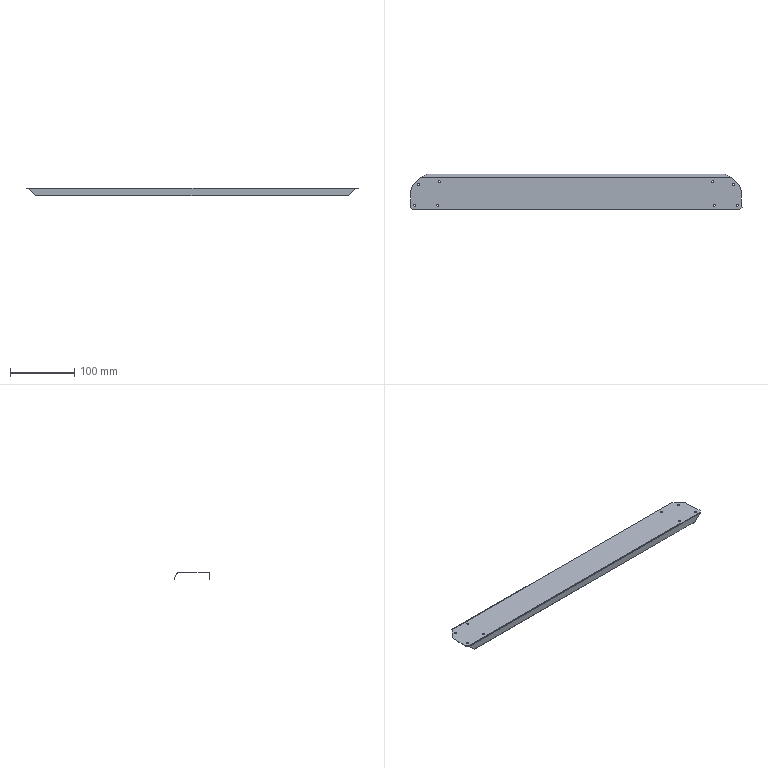Part | SolidWorks | features BaseBody 1 | 1 solid | 42 faces | box 516.336 x 55.923 x 11.911 mm | volume 18267 mm3 | cylinder 20 | plane 18 | spline 4 | commonest cylinder face diameters 3.2 x16 1 x2 2 x2
STEP:
#1=CARTESIAN_POINT('',(252.248,-18.411,-0.5));
#2=VERTEX_POINT('',#1);
#3=CARTESIAN_POINT('',(249.048,-18.411,-0.5));
#4=VERTEX_POINT('',#3);
#5=CARTESIAN_POINT('',(250.648,-18.411,-0.5));
#6=DIRECTION('',(0.,0.,-1.));
#7=DIRECTION('',(1.,0.,0.));
#8=AXIS2_PLACEMENT_3D('',#5,#6,#7);
#9=CIRCLE('',#8,1.6);
#10=EDGE_CURVE('',#2,#4,#9,.T.);
#11=ORIENTED_EDGE('',*,*,#10,.T.);
#12=CARTESIAN_POINT('',(249.048,-18.411,0.));
#13=VERTEX_POINT('',#12);
#14=CARTESIAN_POINT('',(249.048,-18.411,-0.5));
#15=DIRECTION('',(0.,0.,1.));
#16=VECTOR('',#15,1000.);
#17=LINE('',#14,#16);
#18=EDGE_CURVE('',#4,#13,#17,.T.);
#19=ORIENTED_EDGE('',*,*,#18,.T.);
#20=CARTESIAN_POINT('',(252.248,-18.411,0.));
#21=VERTEX_POINT('',#20);
#22=CARTESIAN_POINT('',(250.648,-18.411,0.));
#23=DIRECTION('',(0.,0.,1.));
#24=DIRECTION('',(1.,0.,0.));
#25=AXIS2_PLACEMENT_3D('',#22,#23,#24);
#26=CIRCLE('',#25,1.6);
#27=EDGE_CURVE('',#13,#21,#26,.T.);
#28=ORIENTED_EDGE('',*,*,#27,.T.);
#29=CARTESIAN_POINT('',(252.248,-18.411,-0.5));
#30=DIRECTION('',(0.,0.,1.));
#31=VECTOR('',#30,1000.);
#32=LINE('',#29,#31);
#33=EDGE_CURVE('',#2,#21,#32,.T.);
#34=ORIENTED_EDGE('',*,*,#33,.F.);
#35=EDGE_LOOP('',(#11,#19,#28,#34));
#36=FACE_OUTER_BOUND('',#35,.T.);
#37=CARTESIAN_POINT('',(250.648,-18.411,-0.5));
#38=DIRECTION('',(0.,0.,1.));
#39=DIRECTION('',(1.,0.,0.));
#40=AXIS2_PLACEMENT_3D('',#37,#38,#39);
#41=CYLINDRICAL_SURFACE('',#40,1.6);
#42=ADVANCED_FACE('',(#36),#41,.F.);
#43=CARTESIAN_POINT('',(-252.248,-18.411,-0.5));
#44=VERTEX_POINT('',#43);
#45=CARTESIAN_POINT('',(-249.048,-18.411,-0.5));
#46=VERTEX_POINT('',#45);
#47=CARTESIAN_POINT('',(-250.648,-18.411,-0.5));
#48=DIRECTION('',(0.,0.,1.));
#49=DIRECTION('',(1.,0.,0.));
#50=AXIS2_PLACEMENT_3D('',#47,#48,#49);
#51=CIRCLE('',#50,1.6);
#52=EDGE_CURVE('',#44,#46,#51,.T.);
#53=ORIENTED_EDGE('',*,*,#52,.F.);
#54=CARTESIAN_POINT('',(-252.248,-18.411,0.));
#55=VERTEX_POINT('',#54);
#56=CARTESIAN_POINT('',(-252.248,-18.411,-0.5));
#57=DIRECTION('',(0.,0.,1.));
#58=VECTOR('',#57,1000.);
#59=LINE('',#56,#58);
#60=EDGE_CURVE('',#44,#55,#59,.T.);
#61=ORIENTED_EDGE('',*,*,#60,.T.);
#62=CARTESIAN_POINT('',(-249.048,-18.411,0.));
#63=VERTEX_POINT('',#62);
#64=CARTESIAN_POINT('',(-250.648,-18.411,0.));
#65=DIRECTION('',(0.,0.,1.));
#66=DIRECTION('',(1.,0.,0.));
#67=AXIS2_PLACEMENT_3D('',#64,#65,#66);
#68=CIRCLE('',#67,1.6);
#69=EDGE_CURVE('',#55,#63,#68,.T.);
#70=ORIENTED_EDGE('',*,*,#69,.T.);
#71=CARTESIAN_POINT('',(-249.048,-18.411,-0.5));
#72=DIRECTION('',(0.,0.,1.));
#73=VECTOR('',#72,1000.);
#74=LINE('',#71,#73);
#75=EDGE_CURVE('',#46,#63,#74,.T.);
#76=ORIENTED_EDGE('',*,*,#75,.F.);
#77=EDGE_LOOP('',(#53,#61,#70,#76));
#78=FACE_OUTER_BOUND('',#77,.T.);
#79=CARTESIAN_POINT('',(-250.648,-18.411,-0.5));
#80=DIRECTION('',(0.,0.,1.));
#81=DIRECTION('',(1.,0.,0.));
#82=AXIS2_PLACEMENT_3D('',#79,#80,#81);
#83=CYLINDRICAL_SURFACE('',#82,1.6);
#84=ADVANCED_FACE('',(#78),#83,.F.);
#85=CARTESIAN_POINT('',(-216.439,-18.411,-0.5));
#86=VERTEX_POINT('',#85);
#87=CARTESIAN_POINT('',(-213.239,-18.411,-0.5));
#88=VERTEX_POINT('',#87);
#89=CARTESIAN_POINT('',(-214.839,-18.411,-0.5));
#90=DIRECTION('',(0.,0.,1.));
#91=DIRECTION('',(1.,0.,0.));
#92=AXIS2_PLACEMENT_3D('',#89,#90,#91);
#93=CIRCLE('',#92,1.6);
#94=EDGE_CURVE('',#86,#88,#93,.T.);
#95=ORIENTED_EDGE('',*,*,#94,.F.);
#96=CARTESIAN_POINT('',(-216.439,-18.411,0.));
#97=VERTEX_POINT('',#96);
#98=CARTESIAN_POINT('',(-216.439,-18.411,-0.5));
#99=DIRECTION('',(0.,0.,1.));
#100=VECTOR('',#99,1000.);
#101=LINE('',#98,#100);
#102=EDGE_CURVE('',#86,#97,#101,.T.);
#103=ORIENTED_EDGE('',*,*,#102,.T.);
#104=CARTESIAN_POINT('',(-213.239,-18.411,0.));
#105=VERTEX_POINT('',#104);
#106=CARTESIAN_POINT('',(-214.839,-18.411,0.));
#107=DIRECTION('',(0.,0.,1.));
#108=DIRECTION('',(1.,0.,0.));
#109=AXIS2_PLACEMENT_3D('',#106,#107,#108);
#110=CIRCLE('',#109,1.6);
#111=EDGE_CURVE('',#97,#105,#110,.T.);
#112=ORIENTED_EDGE('',*,*,#111,.T.);
#113=CARTESIAN_POINT('',(-213.239,-18.411,-0.5));
#114=DIRECTION('',(0.,0.,1.));
#115=VECTOR('',#114,1000.);
#116=LINE('',#113,#115);
#117=EDGE_CURVE('',#88,#105,#116,.T.);
#118=ORIENTED_EDGE('',*,*,#117,.F.);
#119=EDGE_LOOP('',(#95,#103,#112,#118));
#120=FACE_OUTER_BOUND('',#119,.T.);
#121=CARTESIAN_POINT('',(-214.839,-18.411,-0.5));
#122=DIRECTION('',(0.,0.,1.));
#123=DIRECTION('',(1.,0.,0.));
#124=AXIS2_PLACEMENT_3D('',#121,#122,#123);
#125=CYLINDRICAL_SURFACE('',#124,1.6);
#126=ADVANCED_FACE('',(#120),#125,.F.);
#127=CARTESIAN_POINT('',(-214.368,18.639,-0.5));
#128=VERTEX_POINT('',#127);
#129=CARTESIAN_POINT('',(-211.168,18.639,-0.5));
#130=VERTEX_POINT('',#129);
#131=CARTESIAN_POINT('',(-212.768,18.639,-0.5));
#132=DIRECTION('',(0.,0.,1.));
#133=DIRECTION('',(1.,0.,0.));
#134=AXIS2_PLACEMENT_3D('',#131,#132,#133);
#135=CIRCLE('',#134,1.6);
#136=EDGE_CURVE('',#128,#130,#135,.T.);
#137=ORIENTED_EDGE('',*,*,#136,.F.);
#138=CARTESIAN_POINT('',(-214.368,18.639,0.));
#139=VERTEX_POINT('',#138);
#140=CARTESIAN_POINT('',(-214.368,18.639,-0.5));
#141=DIRECTION('',(0.,0.,1.));
#142=VECTOR('',#141,1000.);
#143=LINE('',#140,#142);
#144=EDGE_CURVE('',#128,#139,#143,.T.);
#145=ORIENTED_EDGE('',*,*,#144,.T.);
#146=CARTESIAN_POINT('',(-211.168,18.639,0.));
#147=VERTEX_POINT('',#146);
#148=CARTESIAN_POINT('',(-212.768,18.639,0.));
#149=DIRECTION('',(0.,0.,1.));
#150=DIRECTION('',(1.,0.,0.));
#151=AXIS2_PLACEMENT_3D('',#148,#149,#150);
#152=CIRCLE('',#151,1.6);
#153=EDGE_CURVE('',#139,#147,#152,.T.);
#154=ORIENTED_EDGE('',*,*,#153,.T.);
#155=CARTESIAN_POINT('',(-211.168,18.639,-0.5));
#156=DIRECTION('',(0.,0.,1.));
#157=VECTOR('',#156,1000.);
#158=LINE('',#155,#157);
#159=EDGE_CURVE('',#130,#147,#158,.T.);
#160=ORIENTED_EDGE('',*,*,#159,.F.);
#161=EDGE_LOOP('',(#137,#145,#154,#160));
#162=FACE_OUTER_BOUND('',#161,.T.);
#163=CARTESIAN_POINT('',(-212.768,18.639,-0.5));
#164=DIRECTION('',(0.,0.,1.));
#165=DIRECTION('',(1.,0.,0.));
#166=AXIS2_PLACEMENT_3D('',#163,#164,#165);
#167=CYLINDRICAL_SURFACE('',#166,1.6);
#168=ADVANCED_FACE('',(#162),#167,.F.);
#169=CARTESIAN_POINT('',(-246.535,13.819,-0.5));
#170=VERTEX_POINT('',#169);
#171=CARTESIAN_POINT('',(-243.335,13.819,-0.5));
#172=VERTEX_POINT('',#171);
#173=CARTESIAN_POINT('',(-244.935,13.819,-0.5));
#174=DIRECTION('',(0.,0.,1.));
#175=DIRECTION('',(1.,0.,0.));
#176=AXIS2_PLACEMENT_3D('',#173,#174,#175);
#177=CIRCLE('',#176,1.6);
#178=EDGE_CURVE('',#170,#172,#177,.T.);
#179=ORIENTED_EDGE('',*,*,#178,.F.);
#180=CARTESIAN_POINT('',(-246.535,13.819,0.));
#181=VERTEX_POINT('',#180);
#182=CARTESIAN_POINT('',(-246.535,13.819,-0.5));
#183=DIRECTION('',(0.,0.,1.));
#184=VECTOR('',#183,1000.);
#185=LINE('',#182,#184);
#186=EDGE_CURVE('',#170,#181,#185,.T.);
#187=ORIENTED_EDGE('',*,*,#186,.T.);
#188=CARTESIAN_POINT('',(-243.335,13.819,0.));
#189=VERTEX_POINT('',#188);
#190=CARTESIAN_POINT('',(-244.935,13.819,0.));
#191=DIRECTION('',(0.,0.,1.));
#192=DIRECTION('',(1.,0.,0.));
#193=AXIS2_PLACEMENT_3D('',#190,#191,#192);
#194=CIRCLE('',#193,1.6);
#195=EDGE_CURVE('',#181,#189,#194,.T.);
#196=ORIENTED_EDGE('',*,*,#195,.T.);
#197=CARTESIAN_POINT('',(-243.335,13.819,-0.5));
#198=DIRECTION('',(0.,0.,1.));
#199=VECTOR('',#198,1000.);
#200=LINE('',#197,#199);
#201=EDGE_CURVE('',#172,#189,#200,.T.);
#202=ORIENTED_EDGE('',*,*,#201,.F.);
#203=EDGE_LOOP('',(#179,#187,#196,#202));
#204=FACE_OUTER_BOUND('',#203,.T.);
#205=CARTESIAN_POINT('',(-244.935,13.819,-0.5));
#206=DIRECTION('',(0.,0.,1.));
#207=DIRECTION('',(1.,0.,0.));
#208=AXIS2_PLACEMENT_3D('',#205,#206,#207);
#209=CYLINDRICAL_SURFACE('',#208,1.6);
#210=ADVANCED_FACE('',(#204),#209,.F.);
#211=CARTESIAN_POINT('',(213.239,-18.411,-0.5));
#212=VERTEX_POINT('',#211);
#213=CARTESIAN_POINT('',(216.439,-18.411,-0.5));
#214=VERTEX_POINT('',#213);
#215=CARTESIAN_POINT('',(214.839,-18.411,-0.5));
#216=DIRECTION('',(0.,0.,1.));
#217=DIRECTION('',(1.,0.,0.));
#218=AXIS2_PLACEMENT_3D('',#215,#216,#217);
#219=CIRCLE('',#218,1.6);
#220=EDGE_CURVE('',#212,#214,#219,.T.);
#221=ORIENTED_EDGE('',*,*,#220,.F.);
#222=CARTESIAN_POINT('',(213.239,-18.411,0.));
#223=VERTEX_POINT('',#222);
#224=CARTESIAN_POINT('',(213.239,-18.411,-0.5));
#225=DIRECTION('',(0.,0.,1.));
#226=VECTOR('',#225,1000.);
#227=LINE('',#224,#226);
#228=EDGE_CURVE('',#212,#223,#227,.T.);
#229=ORIENTED_EDGE('',*,*,#228,.T.);
#230=CARTESIAN_POINT('',(216.439,-18.411,0.));
#231=VERTEX_POINT('',#230);
#232=CARTESIAN_POINT('',(214.839,-18.411,0.));
#233=DIRECTION('',(0.,0.,1.));
#234=DIRECTION('',(1.,0.,0.));
#235=AXIS2_PLACEMENT_3D('',#232,#233,#234);
#236=CIRCLE('',#235,1.6);
#237=EDGE_CURVE('',#223,#231,#236,.T.);
#238=ORIENTED_EDGE('',*,*,#237,.T.);
#239=CARTESIAN_POINT('',(216.439,-18.411,-0.5));
#240=DIRECTION('',(0.,0.,1.));
#241=VECTOR('',#240,1000.);
#242=LINE('',#239,#241);
#243=EDGE_CURVE('',#214,#231,#242,.T.);
#244=ORIENTED_EDGE('',*,*,#243,.F.);
#245=EDGE_LOOP('',(#221,#229,#238,#244));
#246=FACE_OUTER_BOUND('',#245,.T.);
#247=CARTESIAN_POINT('',(214.839,-18.411,-0.5));
#248=DIRECTION('',(0.,0.,1.));
#249=DIRECTION('',(1.,0.,0.));
#250=AXIS2_PLACEMENT_3D('',#247,#248,#249);
#251=CYLINDRICAL_SURFACE('',#250,1.6);
#252=ADVANCED_FACE('',(#246),#251,.F.);
#253=CARTESIAN_POINT('',(211.168,18.639,-0.5));
#254=VERTEX_POINT('',#253);
#255=CARTESIAN_POINT('',(214.368,18.639,-0.5));
#256=VERTEX_POINT('',#255);
#257=CARTESIAN_POINT('',(212.768,18.639,-0.5));
#258=DIRECTION('',(0.,0.,1.));
#259=DIRECTION('',(1.,0.,0.));
#260=AXIS2_PLACEMENT_3D('',#257,#258,#259);
#261=CIRCLE('',#260,1.6);
#262=EDGE_CURVE('',#254,#256,#261,.T.);
#263=ORIENTED_EDGE('',*,*,#262,.F.);
#264=CARTESIAN_POINT('',(211.168,18.639,0.));
#265=VERTEX_POINT('',#264);
#266=CARTESIAN_POINT('',(211.168,18.639,-0.5));
#267=DIRECTION('',(0.,0.,1.));
#268=VECTOR('',#267,1000.);
#269=LINE('',#266,#268);
#270=EDGE_CURVE('',#254,#265,#269,.T.);
#271=ORIENTED_EDGE('',*,*,#270,.T.);
#272=CARTESIAN_POINT('',(214.368,18.639,0.));
#273=VERTEX_POINT('',#272);
#274=CARTESIAN_POINT('',(212.768,18.639,0.));
#275=DIRECTION('',(0.,0.,1.));
#276=DIRECTION('',(1.,0.,0.));
#277=AXIS2_PLACEMENT_3D('',#274,#275,#276);
#278=CIRCLE('',#277,1.6);
#279=EDGE_CURVE('',#265,#273,#278,.T.);
#280=ORIENTED_EDGE('',*,*,#279,.T.);
#281=CARTESIAN_POINT('',(214.368,18.639,-0.5));
#282=DIRECTION('',(0.,0.,1.));
#283=VECTOR('',#282,1000.);
#284=LINE('',#281,#283);
#285=EDGE_CURVE('',#256,#273,#284,.T.);
#286=ORIENTED_EDGE('',*,*,#285,.F.);
#287=EDGE_LOOP('',(#263,#271,#280,#286));
#288=FACE_OUTER_BOUND('',#287,.T.);
#289=CARTESIAN_POINT('',(212.768,18.639,-0.5));
#290=DIRECTION('',(0.,0.,1.));
#291=DIRECTION('',(1.,0.,0.));
#292=AXIS2_PLACEMENT_3D('',#289,#290,#291);
#293=CYLINDRICAL_SURFACE('',#292,1.6);
#294=ADVANCED_FACE('',(#288),#293,.F.);
#295=CARTESIAN_POINT('',(243.335,13.819,-0.5));
#296=VERTEX_POINT('',#295);
#297=CARTESIAN_POINT('',(246.535,13.819,-0.5));
#298=VERTEX_POINT('',#297);
#299=CARTESIAN_POINT('',(244.935,13.819,-0.5));
#300=DIRECTION('',(0.,0.,1.));
#301=DIRECTION('',(1.,0.,0.));
#302=AXIS2_PLACEMENT_3D('',#299,#300,#301);
#303=CIRCLE('',#302,1.6);
#304=EDGE_CURVE('',#296,#298,#303,.T.);
#305=ORIENTED_EDGE('',*,*,#304,.F.);
#306=CARTESIAN_POINT('',(243.335,13.819,0.));
#307=VERTEX_POINT('',#306);
#308=CARTESIAN_POINT('',(243.335,13.819,-0.5));
#309=DIRECTION('',(0.,0.,1.));
#310=VECTOR('',#309,1000.);
#311=LINE('',#308,#310);
#312=EDGE_CURVE('',#296,#307,#311,.T.);
#313=ORIENTED_EDGE('',*,*,#312,.T.);
#314=CARTESIAN_POINT('',(246.535,13.819,0.));
#315=VERTEX_POINT('',#314);
#316=CARTESIAN_POINT('',(244.935,13.819,0.));
#317=DIRECTION('',(0.,0.,1.));
#318=DIRECTION('',(1.,0.,0.));
#319=AXIS2_PLACEMENT_3D('',#316,#317,#318);
#320=CIRCLE('',#319,1.6);
#321=EDGE_CURVE('',#307,#315,#320,.T.);
#322=ORIENTED_EDGE('',*,*,#321,.T.);
#323=CARTESIAN_POINT('',(246.535,13.819,-0.5));
#324=DIRECTION('',(0.,0.,1.));
#325=VECTOR('',#324,1000.);
#326=LINE('',#323,#325);
#327=EDGE_CURVE('',#298,#315,#326,.T.);
#328=ORIENTED_EDGE('',*,*,#327,.F.);
#329=EDGE_LOOP('',(#305,#313,#322,#328));
#330=FACE_OUTER_BOUND('',#329,.T.);
#331=CARTESIAN_POINT('',(244.935,13.819,-0.5));
#332=DIRECTION('',(0.,0.,1.));
#333=DIRECTION('',(1.,0.,0.));
#334=AXIS2_PLACEMENT_3D('',#331,#332,#333);
#335=CYLINDRICAL_SURFACE('',#334,1.6);
#336=ADVANCED_FACE('',(#330),#335,.F.);
#337=ORIENTED_EDGE('',*,*,#18,.F.);
#338=CARTESIAN_POINT('',(250.648,-18.411,-0.5));
#339=DIRECTION('',(0.,0.,-1.));
#340=DIRECTION('',(1.,0.,0.));
#341=AXIS2_PLACEMENT_3D('',#338,#339,#340);
#342=CIRCLE('',#341,1.6);
#343=EDGE_CURVE('',#4,#2,#342,.T.);
#344=ORIENTED_EDGE('',*,*,#343,.T.);
#345=ORIENTED_EDGE('',*,*,#33,.T.);
#346=CARTESIAN_POINT('',(250.648,-18.411,0.));
#347=DIRECTION('',(0.,0.,1.));
#348=DIRECTION('',(1.,0.,0.));
#349=AXIS2_PLACEMENT_3D('',#346,#347,#348);
#350=CIRCLE('',#349,1.6);
#351=EDGE_CURVE('',#21,#13,#350,.T.);
#352=ORIENTED_EDGE('',*,*,#351,.T.);
#353=EDGE_LOOP('',(#337,#344,#345,#352));
#354=FACE_OUTER_BOUND('',#353,.T.);
#355=CARTESIAN_POINT('',(250.648,-18.411,-0.5));
#356=DIRECTION('',(0.,0.,1.));
#357=DIRECTION('',(1.,0.,0.));
#358=AXIS2_PLACEMENT_3D('',#355,#356,#357);
#359=CYLINDRICAL_SURFACE('',#358,1.6);
#360=ADVANCED_FACE('',(#354),#359,.F.);
#361=CARTESIAN_POINT('',(-250.648,-18.411,0.));
#362=DIRECTION('',(0.,0.,1.));
#363=DIRECTION('',(1.,0.,0.));
#364=AXIS2_PLACEMENT_3D('',#361,#362,#363);
#365=CIRCLE('',#364,1.6);
#366=EDGE_CURVE('',#63,#55,#365,.T.);
#367=ORIENTED_EDGE('',*,*,#366,.F.);
#368=ORIENTED_EDGE('',*,*,#69,.F.);
#369=EDGE_LOOP('',(#367,#368));
#370=FACE_BOUND('',#369,.T.);
#371=CARTESIAN_POINT('',(-214.839,-18.411,0.));
#372=DIRECTION('',(0.,0.,1.));
#373=DIRECTION('',(1.,0.,0.));
#374=AXIS2_PLACEMENT_3D('',#371,#372,#373);
#375=CIRCLE('',#374,1.6);
#376=EDGE_CURVE('',#105,#97,#375,.T.);
#377=ORIENTED_EDGE('',*,*,#376,.F.);
#378=ORIENTED_EDGE('',*,*,#111,.F.);
#379=EDGE_LOOP('',(#377,#378));
#380=FACE_BOUND('',#379,.T.);
#381=CARTESIAN_POINT('',(-212.768,18.639,0.));
#382=DIRECTION('',(0.,0.,1.));
#383=DIRECTION('',(1.,0.,0.));
#384=AXIS2_PLACEMENT_3D('',#381,#382,#383);
#385=CIRCLE('',#384,1.6);
#386=EDGE_CURVE('',#147,#139,#385,.T.);
#387=ORIENTED_EDGE('',*,*,#386,.F.);
#388=ORIENTED_EDGE('',*,*,#153,.F.);
#389=EDGE_LOOP('',(#387,#388));
#390=FACE_BOUND('',#389,.T.);
#391=CARTESIAN_POINT('',(-244.935,13.819,0.));
#392=DIRECTION('',(0.,0.,1.));
#393=DIRECTION('',(1.,0.,0.));
#394=AXIS2_PLACEMENT_3D('',#391,#392,#393);
#395=CIRCLE('',#394,1.6);
#396=EDGE_CURVE('',#189,#181,#395,.T.);
#397=ORIENTED_EDGE('',*,*,#396,.F.);
#398=ORIENTED_EDGE('',*,*,#195,.F.);
#399=EDGE_LOOP('',(#397,#398));
#400=FACE_BOUND('',#399,.T.);
#401=CARTESIAN_POINT('',(214.839,-18.411,0.));
#402=DIRECTION('',(0.,0.,1.));
#403=DIRECTION('',(1.,0.,0.));
#404=AXIS2_PLACEMENT_3D('',#401,#402,#403);
#405=CIRCLE('',#404,1.6);
#406=EDGE_CURVE('',#231,#223,#405,.T.);
#407=ORIENTED_EDGE('',*,*,#406,.F.);
#408=ORIENTED_EDGE('',*,*,#237,.F.);
#409=EDGE_LOOP('',(#407,#408));
#410=FACE_BOUND('',#409,.T.);
#411=CARTESIAN_POINT('',(212.768,18.639,0.));
#412=DIRECTION('',(0.,0.,1.));
#413=DIRECTION('',(1.,0.,0.));
#414=AXIS2_PLACEMENT_3D('',#411,#412,#413);
#415=CIRCLE('',#414,1.6);
#416=EDGE_CURVE('',#273,#265,#415,.T.);
#417=ORIENTED_EDGE('',*,*,#416,.F.);
#418=ORIENTED_EDGE('',*,*,#279,.F.);
#419=EDGE_LOOP('',(#417,#418));
#420=FACE_BOUND('',#419,.T.);
#421=CARTESIAN_POINT('',(244.935,13.819,0.));
#422=DIRECTION('',(0.,0.,1.));
#423=DIRECTION('',(1.,0.,0.));
#424=AXIS2_PLACEMENT_3D('',#421,#422,#423);
#425=CIRCLE('',#424,1.6);
#426=EDGE_CURVE('',#315,#307,#425,.T.);
#427=ORIENTED_EDGE('',*,*,#426,.F.);
#428=ORIENTED_EDGE('',*,*,#321,.F.);
#429=EDGE_LOOP('',(#427,#428));
#430=FACE_BOUND('',#429,.T.);
#431=ORIENTED_EDGE('',*,*,#351,.F.);
#432=ORIENTED_EDGE('',*,*,#27,.F.);
#433=EDGE_LOOP('',(#431,#432));
#434=FACE_BOUND('',#433,.T.);
#435=CARTESIAN_POINT('',(-256.428,9.,0.));
#436=VERTEX_POINT('',#435);
#437=CARTESIAN_POINT('',(-241.892,24.588,0.));
#438=VERTEX_POINT('',#437);
#439=CARTESIAN_POINT('',(-241.892,24.588,0.));
#440=DIRECTION('',(0.682,0.7314,0.));
#441=VECTOR('',#440,1000.);
#442=LINE('',#439,#441);
#443=EDGE_CURVE('',#436,#438,#442,.T.);
#444=ORIENTED_EDGE('',*,*,#443,.F.);
#445=CARTESIAN_POINT('',(-258.168,-21.,0.));
#446=VERTEX_POINT('',#445);
#447=CARTESIAN_POINT('',(-256.428,9.,0.));
#448=DIRECTION('',(0.0579,0.9983,0.));
#449=VECTOR('',#448,1000.);
#450=LINE('',#447,#449);
#451=EDGE_CURVE('',#446,#436,#450,.T.);
#452=ORIENTED_EDGE('',*,*,#451,.F.);
#453=CARTESIAN_POINT('',(-254.757,-24.411,0.));
#454=VERTEX_POINT('',#453);
#455=CARTESIAN_POINT('',(-258.168,-21.,0.));
#456=DIRECTION('',(-0.7071,0.7071,0.));
#457=VECTOR('',#456,1000.);
#458=LINE('',#455,#457);
#459=EDGE_CURVE('',#454,#446,#458,.T.);
#460=ORIENTED_EDGE('',*,*,#459,.F.);
#461=CARTESIAN_POINT('',(254.757,-24.411,0.));
#462=VERTEX_POINT('',#461);
#463=CARTESIAN_POINT('',(0.,-24.411,0.));
#464=DIRECTION('',(-1.,0.,0.));
#465=VECTOR('',#464,1000.);
#466=LINE('',#463,#465);
#467=EDGE_CURVE('',#462,#454,#466,.T.);
#468=ORIENTED_EDGE('',*,*,#467,.F.);
#469=CARTESIAN_POINT('',(258.168,-21.,0.));
#470=VERTEX_POINT('',#469);
#471=CARTESIAN_POINT('',(254.757,-24.411,0.));
#472=DIRECTION('',(-0.7071,-0.7071,0.));
#473=VECTOR('',#472,1000.);
#474=LINE('',#471,#473);
#475=EDGE_CURVE('',#470,#462,#474,.T.);
#476=ORIENTED_EDGE('',*,*,#475,.F.);
#477=CARTESIAN_POINT('',(256.428,9.,0.));
#478=VERTEX_POINT('',#477);
#479=CARTESIAN_POINT('',(258.168,-21.,0.));
#480=DIRECTION('',(0.0579,-0.9983,0.));
#481=VECTOR('',#480,1000.);
#482=LINE('',#479,#481);
#483=EDGE_CURVE('',#478,#470,#482,.T.);
#484=ORIENTED_EDGE('',*,*,#483,.F.);
#485=CARTESIAN_POINT('',(241.892,24.588,0.));
#486=VERTEX_POINT('',#485);
#487=CARTESIAN_POINT('',(256.428,9.,0.));
#488=DIRECTION('',(0.682,-0.7314,0.));
#489=VECTOR('',#488,1000.);
#490=LINE('',#487,#489);
#491=EDGE_CURVE('',#486,#478,#490,.T.);
#492=ORIENTED_EDGE('',*,*,#491,.F.);
#493=CARTESIAN_POINT('',(0.,24.588,0.));
#494=DIRECTION('',(1.,0.,0.));
#495=VECTOR('',#494,1000.);
#496=LINE('',#493,#495);
#497=EDGE_CURVE('',#438,#486,#496,.T.);
#498=ORIENTED_EDGE('',*,*,#497,.F.);
#499=EDGE_LOOP('',(#444,#452,#460,#468,#476,#484,#492,#498));
#500=FACE_OUTER_BOUND('',#499,.T.);
#501=CARTESIAN_POINT('',(261.266,-24.411,0.));
#502=DIRECTION('',(0.,0.,-1.));
#503=DIRECTION('',(-1.,0.,0.));
#504=AXIS2_PLACEMENT_3D('',#501,#502,#503);
#505=PLANE('',#504);
#506=ADVANCED_FACE('',(#370,#380,#390,#400,#410,#420,#430,#434,#500),#505,.F.);
#507=CARTESIAN_POINT('',(-250.648,-18.411,-0.5));
#508=DIRECTION('',(0.,0.,1.));
#509=DIRECTION('',(1.,0.,0.));
#510=AXIS2_PLACEMENT_3D('',#507,#508,#509);
#511=CIRCLE('',#510,1.6);
#512=EDGE_CURVE('',#46,#44,#511,.T.);
#513=ORIENTED_EDGE('',*,*,#512,.T.);
#514=ORIENTED_EDGE('',*,*,#52,.T.);
#515=EDGE_LOOP('',(#513,#514));
#516=FACE_BOUND('',#515,.T.);
#517=CARTESIAN_POINT('',(-214.839,-18.411,-0.5));
#518=DIRECTION('',(0.,0.,1.));
#519=DIRECTION('',(1.,0.,0.));
#520=AXIS2_PLACEMENT_3D('',#517,#518,#519);
#521=CIRCLE('',#520,1.6);
#522=EDGE_CURVE('',#88,#86,#521,.T.);
#523=ORIENTED_EDGE('',*,*,#522,.T.);
#524=ORIENTED_EDGE('',*,*,#94,.T.);
#525=EDGE_LOOP('',(#523,#524));
#526=FACE_BOUND('',#525,.T.);
#527=CARTESIAN_POINT('',(-212.768,18.639,-0.5));
#528=DIRECTION('',(0.,0.,1.));
#529=DIRECTION('',(1.,0.,0.));
#530=AXIS2_PLACEMENT_3D('',#527,#528,#529);
#531=CIRCLE('',#530,1.6);
#532=EDGE_CURVE('',#130,#128,#531,.T.);
#533=ORIENTED_EDGE('',*,*,#532,.T.);
#534=ORIENTED_EDGE('',*,*,#136,.T.);
#535=EDGE_LOOP('',(#533,#534));
#536=FACE_BOUND('',#535,.T.);
#537=CARTESIAN_POINT('',(-244.935,13.819,-0.5));
#538=DIRECTION('',(0.,0.,1.));
#539=DIRECTION('',(1.,0.,0.));
#540=AXIS2_PLACEMENT_3D('',#537,#538,#539);
#541=CIRCLE('',#540,1.6);
#542=EDGE_CURVE('',#172,#170,#541,.T.);
#543=ORIENTED_EDGE('',*,*,#542,.T.);
#544=ORIENTED_EDGE('',*,*,#178,.T.);
#545=EDGE_LOOP('',(#543,#544));
#546=FACE_BOUND('',#545,.T.);
#547=CARTESIAN_POINT('',(214.839,-18.411,-0.5));
#548=DIRECTION('',(0.,0.,1.));
#549=DIRECTION('',(1.,0.,0.));
#550=AXIS2_PLACEMENT_3D('',#547,#548,#549);
#551=CIRCLE('',#550,1.6);
#552=EDGE_CURVE('',#214,#212,#551,.T.);
#553=ORIENTED_EDGE('',*,*,#552,.T.);
#554=ORIENTED_EDGE('',*,*,#220,.T.);
#555=EDGE_LOOP('',(#553,#554));
#556=FACE_BOUND('',#555,.T.);
#557=CARTESIAN_POINT('',(212.768,18.639,-0.5));
#558=DIRECTION('',(0.,0.,1.));
#559=DIRECTION('',(1.,0.,0.));
#560=AXIS2_PLACEMENT_3D('',#557,#558,#559);
#561=CIRCLE('',#560,1.6);
#562=EDGE_CURVE('',#256,#254,#561,.T.);
#563=ORIENTED_EDGE('',*,*,#562,.T.);
#564=ORIENTED_EDGE('',*,*,#262,.T.);
#565=EDGE_LOOP('',(#563,#564));
#566=FACE_BOUND('',#565,.T.);
#567=CARTESIAN_POINT('',(244.935,13.819,-0.5));
#568=DIRECTION('',(0.,0.,1.));
#569=DIRECTION('',(1.,0.,0.));
#570=AXIS2_PLACEMENT_3D('',#567,#568,#569);
#571=CIRCLE('',#570,1.6);
#572=EDGE_CURVE('',#298,#296,#571,.T.);
#573=ORIENTED_EDGE('',*,*,#572,.T.);
#574=ORIENTED_EDGE('',*,*,#304,.T.);
#575=EDGE_LOOP('',(#573,#574));
#576=FACE_BOUND('',#575,.T.);
#577=ORIENTED_EDGE('',*,*,#10,.F.);
#578=ORIENTED_EDGE('',*,*,#343,.F.);
#579=EDGE_LOOP('',(#577,#578));
#580=FACE_BOUND('',#579,.T.);
#581=CARTESIAN_POINT('',(-254.757,-24.411,-0.5));
#582=VERTEX_POINT('',#581);
#583=CARTESIAN_POINT('',(-258.168,-21.,-0.5));
#584=VERTEX_POINT('',#583);
#585=CARTESIAN_POINT('',(-254.757,-24.411,-0.5));
#586=DIRECTION('',(-0.7071,0.7071,0.));
#587=VECTOR('',#586,1000.);
#588=LINE('',#585,#587);
#589=EDGE_CURVE('',#582,#584,#588,.T.);
#590=ORIENTED_EDGE('',*,*,#589,.T.);
#591=CARTESIAN_POINT('',(-256.428,9.,-0.5));
#592=VERTEX_POINT('',#591);
#593=CARTESIAN_POINT('',(-258.168,-21.,-0.5));
#594=DIRECTION('',(0.0579,0.9983,0.));
#595=VECTOR('',#594,1000.);
#596=LINE('',#593,#595);
#597=EDGE_CURVE('',#584,#592,#596,.T.);
#598=ORIENTED_EDGE('',*,*,#597,.T.);
#599=CARTESIAN_POINT('',(-241.892,24.588,-0.5));
#600=VERTEX_POINT('',#599);
#601=CARTESIAN_POINT('',(-256.428,9.,-0.5));
#602=DIRECTION('',(0.682,0.7314,0.));
#603=VECTOR('',#602,1000.);
#604=LINE('',#601,#603);
#605=EDGE_CURVE('',#592,#600,#604,.T.);
#606=ORIENTED_EDGE('',*,*,#605,.T.);
#607=CARTESIAN_POINT('',(241.892,24.588,-0.5));
#608=VERTEX_POINT('',#607);
#609=CARTESIAN_POINT('',(0.,24.588,-0.5));
#610=DIRECTION('',(1.,0.,0.));
#611=VECTOR('',#610,1000.);
#612=LINE('',#609,#611);
#613=EDGE_CURVE('',#600,#608,#612,.T.);
#614=ORIENTED_EDGE('',*,*,#613,.T.);
#615=CARTESIAN_POINT('',(256.428,9.,-0.5));
#616=VERTEX_POINT('',#615);
#617=CARTESIAN_POINT('',(241.892,24.588,-0.5));
#618=DIRECTION('',(0.682,-0.7314,0.));
#619=VECTOR('',#618,1000.);
#620=LINE('',#617,#619);
#621=EDGE_CURVE('',#608,#616,#620,.T.);
#622=ORIENTED_EDGE('',*,*,#621,.T.);
#623=CARTESIAN_POINT('',(258.168,-21.,-0.5));
#624=VERTEX_POINT('',#623);
#625=CARTESIAN_POINT('',(256.428,9.,-0.5));
#626=DIRECTION('',(0.0579,-0.9983,0.));
#627=VECTOR('',#626,1000.);
#628=LINE('',#625,#627);
#629=EDGE_CURVE('',#616,#624,#628,.T.);
#630=ORIENTED_EDGE('',*,*,#629,.T.);
#631=CARTESIAN_POINT('',(254.757,-24.411,-0.5));
#632=VERTEX_POINT('',#631);
#633=CARTESIAN_POINT('',(258.168,-21.,-0.5));
#634=DIRECTION('',(-0.7071,-0.7071,0.));
#635=VECTOR('',#634,1000.);
#636=LINE('',#633,#635);
#637=EDGE_CURVE('',#624,#632,#636,.T.);
#638=ORIENTED_EDGE('',*,*,#637,.T.);
#639=CARTESIAN_POINT('',(0.,-24.411,-0.5));
#640=DIRECTION('',(-1.,0.,0.));
#641=VECTOR('',#640,1000.);
#642=LINE('',#639,#641);
#643=EDGE_CURVE('',#632,#582,#642,.T.);
#644=ORIENTED_EDGE('',*,*,#643,.T.);
#645=EDGE_LOOP('',(#590,#598,#606,#614,#622,#630,#638,#644));
#646=FACE_OUTER_BOUND('',#645,.T.);
#647=CARTESIAN_POINT('',(261.266,-24.411,-0.5));
#648=DIRECTION('',(0.,0.,-1.));
#649=DIRECTION('',(-1.,0.,0.));
#650=AXIS2_PLACEMENT_3D('',#647,#648,#649);
#651=PLANE('',#650);
#652=ADVANCED_FACE('',(#516,#526,#536,#546,#556,#566,#576,#580,#646),#651,.T.);
#653=ORIENTED_EDGE('',*,*,#60,.F.);
#654=ORIENTED_EDGE('',*,*,#512,.F.);
#655=ORIENTED_EDGE('',*,*,#75,.T.);
#656=ORIENTED_EDGE('',*,*,#366,.T.);
#657=EDGE_LOOP('',(#653,#654,#655,#656));
#658=FACE_OUTER_BOUND('',#657,.T.);
#659=CARTESIAN_POINT('',(-250.648,-18.411,-0.5));
#660=DIRECTION('',(0.,0.,1.));
#661=DIRECTION('',(1.,0.,0.));
#662=AXIS2_PLACEMENT_3D('',#659,#660,#661);
#663=CYLINDRICAL_SURFACE('',#662,1.6);
#664=ADVANCED_FACE('',(#658),#663,.F.);
#665=ORIENTED_EDGE('',*,*,#102,.F.);
#666=ORIENTED_EDGE('',*,*,#522,.F.);
#667=ORIENTED_EDGE('',*,*,#117,.T.);
#668=ORIENTED_EDGE('',*,*,#376,.T.);
#669=EDGE_LOOP('',(#665,#666,#667,#668));
#670=FACE_OUTER_BOUND('',#669,.T.);
#671=CARTESIAN_POINT('',(-214.839,-18.411,-0.5));
#672=DIRECTION('',(0.,0.,1.));
#673=DIRECTION('',(1.,0.,0.));
#674=AXIS2_PLACEMENT_3D('',#671,#672,#673);
#675=CYLINDRICAL_SURFACE('',#674,1.6);
#676=ADVANCED_FACE('',(#670),#675,.F.);
#677=ORIENTED_EDGE('',*,*,#144,.F.);
#678=ORIENTED_EDGE('',*,*,#532,.F.);
#679=ORIENTED_EDGE('',*,*,#159,.T.);
#680=ORIENTED_EDGE('',*,*,#386,.T.);
#681=EDGE_LOOP('',(#677,#678,#679,#680));
#682=FACE_OUTER_BOUND('',#681,.T.);
#683=CARTESIAN_POINT('',(-212.768,18.639,-0.5));
#684=DIRECTION('',(0.,0.,1.));
#685=DIRECTION('',(1.,0.,0.));
#686=AXIS2_PLACEMENT_3D('',#683,#684,#685);
#687=CYLINDRICAL_SURFACE('',#686,1.6);
#688=ADVANCED_FACE('',(#682),#687,.F.);
#689=ORIENTED_EDGE('',*,*,#186,.F.);
#690=ORIENTED_EDGE('',*,*,#542,.F.);
#691=ORIENTED_EDGE('',*,*,#201,.T.);
#692=ORIENTED_EDGE('',*,*,#396,.T.);
#693=EDGE_LOOP('',(#689,#690,#691,#692));
#694=FACE_OUTER_BOUND('',#693,.T.);
#695=CARTESIAN_POINT('',(-244.935,13.819,-0.5));
#696=DIRECTION('',(0.,0.,1.));
#697=DIRECTION('',(1.,0.,0.));
#698=AXIS2_PLACEMENT_3D('',#695,#696,#697);
#699=CYLINDRICAL_SURFACE('',#698,1.6);
#700=ADVANCED_FACE('',(#694),#699,.F.);
#701=ORIENTED_EDGE('',*,*,#228,.F.);
#702=ORIENTED_EDGE('',*,*,#552,.F.);
#703=ORIENTED_EDGE('',*,*,#243,.T.);
#704=ORIENTED_EDGE('',*,*,#406,.T.);
#705=EDGE_LOOP('',(#701,#702,#703,#704));
#706=FACE_OUTER_BOUND('',#705,.T.);
#707=CARTESIAN_POINT('',(214.839,-18.411,-0.5));
#708=DIRECTION('',(0.,0.,1.));
#709=DIRECTION('',(1.,0.,0.));
#710=AXIS2_PLACEMENT_3D('',#707,#708,#709);
#711=CYLINDRICAL_SURFACE('',#710,1.6);
#712=ADVANCED_FACE('',(#706),#711,.F.);
#713=ORIENTED_EDGE('',*,*,#270,.F.);
#714=ORIENTED_EDGE('',*,*,#562,.F.);
#715=ORIENTED_EDGE('',*,*,#285,.T.);
#716=ORIENTED_EDGE('',*,*,#416,.T.);
#717=EDGE_LOOP('',(#713,#714,#715,#716));
#718=FACE_OUTER_BOUND('',#717,.T.);
#719=CARTESIAN_POINT('',(212.768,18.639,-0.5));
#720=DIRECTION('',(0.,0.,1.));
#721=DIRECTION('',(1.,0.,0.));
#722=AXIS2_PLACEMENT_3D('',#719,#720,#721);
#723=CYLINDRICAL_SURFACE('',#722,1.6);
#724=ADVANCED_FACE('',(#718),#723,.F.);
#725=ORIENTED_EDGE('',*,*,#312,.F.);
#726=ORIENTED_EDGE('',*,*,#572,.F.);
#727=ORIENTED_EDGE('',*,*,#327,.T.);
#728=ORIENTED_EDGE('',*,*,#426,.T.);
#729=EDGE_LOOP('',(#725,#726,#727,#728));
#730=FACE_OUTER_BOUND('',#729,.T.);
#731=CARTESIAN_POINT('',(244.935,13.819,-0.5));
#732=DIRECTION('',(0.,0.,1.));
#733=DIRECTION('',(1.,0.,0.));
#734=AXIS2_PLACEMENT_3D('',#731,#732,#733);
#735=CYLINDRICAL_SURFACE('',#734,1.6);
#736=ADVANCED_FACE('',(#730),#735,.F.);
#737=CARTESIAN_POINT('',(-241.123,25.479,-0.546));
#738=VERTEX_POINT('',#737);
#739=CARTESIAN_POINT('',(-241.892,24.588,0.));
#740=CARTESIAN_POINT('',(-241.828,24.68,-0.000000003));
#741=CARTESIAN_POINT('',(-241.764,24.771,-0.01266));
#742=CARTESIAN_POINT('',(-241.637,24.946,-0.06207));
#743=CARTESIAN_POINT('',(-241.572,25.032,-0.09951));
#744=CARTESIAN_POINT('',(-241.38,25.265,-0.2424));
#745=CARTESIAN_POINT('',(-241.252,25.395,-0.3814));
#746=CARTESIAN_POINT('',(-241.123,25.479,-0.546));
#747=B_SPLINE_CURVE_WITH_KNOTS('',3,(#739,#740,#741,#742,#743,#744,#745,#746),.UNSPECIFIED.,.F.,.F.,(4,2,2,4),(0.,0.0003334,0.0006668,0.001334),.UNSPECIFIED.);
#748=EDGE_CURVE('',#438,#738,#747,.T.);
#749=ORIENTED_EDGE('',*,*,#748,.F.);
#750=ORIENTED_EDGE('',*,*,#497,.T.);
#751=CARTESIAN_POINT('',(241.123,25.479,-0.546));
#752=VERTEX_POINT('',#751);
#753=CARTESIAN_POINT('',(241.123,25.479,-0.546));
#754=CARTESIAN_POINT('',(241.188,25.437,-0.4637));
#755=CARTESIAN_POINT('',(241.251,25.384,-0.3887));
#756=CARTESIAN_POINT('',(241.379,25.261,-0.2546));
#757=CARTESIAN_POINT('',(241.444,25.188,-0.1953));
#758=CARTESIAN_POINT('',(241.635,24.955,-0.0522));
#759=CARTESIAN_POINT('',(241.763,24.772,-0.000000006));
#760=CARTESIAN_POINT('',(241.892,24.588,0.));
#761=B_SPLINE_CURVE_WITH_KNOTS('',3,(#753,#754,#755,#756,#757,#758,#759,#760),.UNSPECIFIED.,.F.,.F.,(4,2,2,4),(0.,0.0003334,0.0006668,0.001334),.UNSPECIFIED.);
#762=EDGE_CURVE('',#752,#486,#761,.T.);
#763=ORIENTED_EDGE('',*,*,#762,.F.);
#764=CARTESIAN_POINT('',(0.,25.479,-0.546));
#765=DIRECTION('',(1.,0.,0.));
#766=VECTOR('',#765,1000.);
#767=LINE('',#764,#766);
#768=EDGE_CURVE('',#738,#752,#767,.T.);
#769=ORIENTED_EDGE('',*,*,#768,.F.);
#770=EDGE_LOOP('',(#749,#750,#763,#769));
#771=FACE_OUTER_BOUND('',#770,.T.);
#772=CARTESIAN_POINT('',(-244.795,24.588,-1.));
#773=DIRECTION('',(1.,0.,0.));
#774=DIRECTION('',(0.,0.,-1.));
#775=AXIS2_PLACEMENT_3D('',#772,#773,#774);
#776=CYLINDRICAL_SURFACE('',#775,1.);
#777=ADVANCED_FACE('',(#771),#776,.T.);
#778=ORIENTED_EDGE('',*,*,#605,.F.);
#779=CARTESIAN_POINT('',(-256.428,9.,-0.25));
#780=DIRECTION('',(0.,0.,1.));
#781=VECTOR('',#780,1000.);
#782=LINE('',#779,#781);
#783=EDGE_CURVE('',#592,#436,#782,.T.);
#784=ORIENTED_EDGE('',*,*,#783,.T.);
#785=ORIENTED_EDGE('',*,*,#443,.T.);
#786=CARTESIAN_POINT('',(-241.892,24.588,-0.25));
#787=DIRECTION('',(0.,0.,-1.));
#788=VECTOR('',#787,1000.);
#789=LINE('',#786,#788);
#790=EDGE_CURVE('',#438,#600,#789,.T.);
#791=ORIENTED_EDGE('',*,*,#790,.T.);
#792=EDGE_LOOP('',(#778,#784,#785,#791));
#793=FACE_OUTER_BOUND('',#792,.T.);
#794=CARTESIAN_POINT('',(-241.892,24.588,-0.5));
#795=DIRECTION('',(-0.7314,0.682,0.));
#796=DIRECTION('',(-0.682,-0.7314,0.));
#797=AXIS2_PLACEMENT_3D('',#794,#795,#796);
#798=PLANE('',#797);
#799=ADVANCED_FACE('',(#793),#798,.T.);
#800=ORIENTED_EDGE('',*,*,#597,.F.);
#801=CARTESIAN_POINT('',(-258.168,-21.,-0.25));
#802=DIRECTION('',(0.,0.,1.));
#803=VECTOR('',#802,1000.);
#804=LINE('',#801,#803);
#805=EDGE_CURVE('',#584,#446,#804,.T.);
#806=ORIENTED_EDGE('',*,*,#805,.T.);
#807=ORIENTED_EDGE('',*,*,#451,.T.);
#808=ORIENTED_EDGE('',*,*,#783,.F.);
#809=EDGE_LOOP('',(#800,#806,#807,#808));
#810=FACE_OUTER_BOUND('',#809,.T.);
#811=CARTESIAN_POINT('',(-256.428,9.,-0.5));
#812=DIRECTION('',(-0.9983,0.0579,0.));
#813=DIRECTION('',(-0.0579,-0.9983,0.));
#814=AXIS2_PLACEMENT_3D('',#811,#812,#813);
#815=PLANE('',#814);
#816=ADVANCED_FACE('',(#810),#815,.T.);
#817=ORIENTED_EDGE('',*,*,#805,.F.);
#818=ORIENTED_EDGE('',*,*,#589,.F.);
#819=CARTESIAN_POINT('',(-254.757,-24.411,-0.25));
#820=DIRECTION('',(0.,0.,1.));
#821=VECTOR('',#820,1000.);
#822=LINE('',#819,#821);
#823=EDGE_CURVE('',#582,#454,#822,.T.);
#824=ORIENTED_EDGE('',*,*,#823,.T.);
#825=ORIENTED_EDGE('',*,*,#459,.T.);
#826=EDGE_LOOP('',(#817,#818,#824,#825));
#827=FACE_OUTER_BOUND('',#826,.T.);
#828=CARTESIAN_POINT('',(-258.168,-21.,-0.5));
#829=DIRECTION('',(-0.7071,-0.7071,0.));
#830=DIRECTION('',(0.7071,-0.7071,0.));
#831=AXIS2_PLACEMENT_3D('',#828,#829,#830);
#832=PLANE('',#831);
#833=ADVANCED_FACE('',(#827),#832,.T.);
#834=CARTESIAN_POINT('',(-253.579,-25.411,-1.));
#835=VERTEX_POINT('',#834);
#836=CARTESIAN_POINT('',(-253.579,-25.411,-1.));
#837=CARTESIAN_POINT('',(-253.678,-25.411,-0.868));
#838=CARTESIAN_POINT('',(-253.774,-25.385,-0.7393));
#839=CARTESIAN_POINT('',(-253.972,-25.285,-0.4959));
#840=CARTESIAN_POINT('',(-254.069,-25.211,-0.3864));
#841=CARTESIAN_POINT('',(-254.364,-24.933,-0.1077));
#842=CARTESIAN_POINT('',(-254.559,-24.675,-0.000000002));
#843=CARTESIAN_POINT('',(-254.757,-24.411,0.));
#844=B_SPLINE_CURVE_WITH_KNOTS('',3,(#836,#837,#838,#839,#840,#841,#842,#843),.UNSPECIFIED.,.F.,.F.,(4,2,2,4),(0.,0.0004884,0.0009769,0.001954),.UNSPECIFIED.);
#845=EDGE_CURVE('',#835,#454,#844,.T.);
#846=ORIENTED_EDGE('',*,*,#845,.F.);
#847=CARTESIAN_POINT('',(253.579,-25.411,-1.));
#848=VERTEX_POINT('',#847);
#849=CARTESIAN_POINT('',(0.,-25.411,-1.));
#850=DIRECTION('',(-1.,0.,0.));
#851=VECTOR('',#850,1000.);
#852=LINE('',#849,#851);
#853=EDGE_CURVE('',#848,#835,#852,.T.);
#854=ORIENTED_EDGE('',*,*,#853,.F.);
#855=CARTESIAN_POINT('',(254.757,-24.411,0.));
#856=CARTESIAN_POINT('',(254.658,-24.543,-0.000000001));
#857=CARTESIAN_POINT('',(254.562,-24.672,-0.02563));
#858=CARTESIAN_POINT('',(254.364,-24.915,-0.1264));
#859=CARTESIAN_POINT('',(254.267,-25.025,-0.1995));
#860=CARTESIAN_POINT('',(253.972,-25.303,-0.4777));
#861=CARTESIAN_POINT('',(253.777,-25.411,-0.736));
#862=CARTESIAN_POINT('',(253.579,-25.411,-1.));
#863=B_SPLINE_CURVE_WITH_KNOTS('',3,(#855,#856,#857,#858,#859,#860,#861,#862),.UNSPECIFIED.,.F.,.F.,(4,2,2,4),(0.,0.0004884,0.0009769,0.001954),.UNSPECIFIED.);
#864=EDGE_CURVE('',#462,#848,#863,.T.);
#865=ORIENTED_EDGE('',*,*,#864,.F.);
#866=ORIENTED_EDGE('',*,*,#467,.T.);
#867=EDGE_LOOP('',(#846,#854,#865,#866));
#868=FACE_OUTER_BOUND('',#867,.T.);
#869=CARTESIAN_POINT('',(257.814,-24.411,-1.));
#870=DIRECTION('',(-1.,0.,0.));
#871=DIRECTION('',(0.,0.,1.));
#872=AXIS2_PLACEMENT_3D('',#869,#870,#871);
#873=CYLINDRICAL_SURFACE('',#872,1.);
#874=ADVANCED_FACE('',(#868),#873,.T.);
#875=CARTESIAN_POINT('',(258.168,-21.,-0.25));
#876=DIRECTION('',(0.,0.,1.));
#877=VECTOR('',#876,1000.);
#878=LINE('',#875,#877);
#879=EDGE_CURVE('',#624,#470,#878,.T.);
#880=ORIENTED_EDGE('',*,*,#879,.T.);
#881=ORIENTED_EDGE('',*,*,#475,.T.);
#882=CARTESIAN_POINT('',(254.757,-24.411,-0.25));
#883=DIRECTION('',(0.,0.,-1.));
#884=VECTOR('',#883,1000.);
#885=LINE('',#882,#884);
#886=EDGE_CURVE('',#462,#632,#885,.T.);
#887=ORIENTED_EDGE('',*,*,#886,.T.);
#888=ORIENTED_EDGE('',*,*,#637,.F.);
#889=EDGE_LOOP('',(#880,#881,#887,#888));
#890=FACE_OUTER_BOUND('',#889,.T.);
#891=CARTESIAN_POINT('',(254.757,-24.411,-0.5));
#892=DIRECTION('',(0.7071,-0.7071,0.));
#893=DIRECTION('',(0.7071,0.7071,0.));
#894=AXIS2_PLACEMENT_3D('',#891,#892,#893);
#895=PLANE('',#894);
#896=ADVANCED_FACE('',(#890),#895,.T.);
#897=ORIENTED_EDGE('',*,*,#629,.F.);
#898=CARTESIAN_POINT('',(256.428,9.,-0.25));
#899=DIRECTION('',(0.,0.,1.));
#900=VECTOR('',#899,1000.);
#901=LINE('',#898,#900);
#902=EDGE_CURVE('',#616,#478,#901,.T.);
#903=ORIENTED_EDGE('',*,*,#902,.T.);
#904=ORIENTED_EDGE('',*,*,#483,.T.);
#905=ORIENTED_EDGE('',*,*,#879,.F.);
#906=EDGE_LOOP('',(#897,#903,#904,#905));
#907=FACE_OUTER_BOUND('',#906,.T.);
#908=CARTESIAN_POINT('',(258.168,-21.,-0.5));
#909=DIRECTION('',(0.9983,0.0579,0.));
#910=DIRECTION('',(-0.0579,0.9983,0.));
#911=AXIS2_PLACEMENT_3D('',#908,#909,#910);
#912=PLANE('',#911);
#913=ADVANCED_FACE('',(#907),#912,.T.);
#914=ORIENTED_EDGE('',*,*,#491,.T.);
#915=ORIENTED_EDGE('',*,*,#902,.F.);
#916=ORIENTED_EDGE('',*,*,#621,.F.);
#917=CARTESIAN_POINT('',(241.892,24.588,-0.25));
#918=DIRECTION('',(0.,0.,1.));
#919=VECTOR('',#918,1000.);
#920=LINE('',#917,#919);
#921=EDGE_CURVE('',#608,#486,#920,.T.);
#922=ORIENTED_EDGE('',*,*,#921,.T.);
#923=EDGE_LOOP('',(#914,#915,#916,#922));
#924=FACE_OUTER_BOUND('',#923,.T.);
#925=CARTESIAN_POINT('',(256.428,9.,-0.5));
#926=DIRECTION('',(0.7314,0.682,0.));
#927=DIRECTION('',(-0.682,0.7314,0.));
#928=AXIS2_PLACEMENT_3D('',#925,#926,#927);
#929=PLANE('',#928);
#930=ADVANCED_FACE('',(#924),#929,.T.);
#931=CARTESIAN_POINT('',(253.579,-24.911,-1.));
#932=VERTEX_POINT('',#931);
#933=CARTESIAN_POINT('',(-253.579,-24.911,-1.));
#934=VERTEX_POINT('',#933);
#935=CARTESIAN_POINT('',(0.,-24.911,-1.));
#936=DIRECTION('',(-1.,0.,0.));
#937=VECTOR('',#936,1000.);
#938=LINE('',#935,#937);
#939=EDGE_CURVE('',#932,#934,#938,.T.);
#940=ORIENTED_EDGE('',*,*,#939,.T.);
#941=CARTESIAN_POINT('',(-253.579,-24.911,-1.));
#942=CARTESIAN_POINT('',(-253.678,-24.911,-0.9341));
#943=CARTESIAN_POINT('',(-253.775,-24.898,-0.8692));
#944=CARTESIAN_POINT('',(-253.971,-24.848,-0.7486));
#945=CARTESIAN_POINT('',(-254.07,-24.811,-0.6926));
#946=CARTESIAN_POINT('',(-254.363,-24.673,-0.5545));
#947=CARTESIAN_POINT('',(-254.559,-24.543,-0.5));
#948=CARTESIAN_POINT('',(-254.757,-24.411,-0.5));
#949=B_SPLINE_CURVE_WITH_KNOTS('',3,(#941,#942,#943,#944,#945,#946,#947,#948),.UNSPECIFIED.,.F.,.F.,(4,2,2,4),(0.,0.0003524,0.0007048,0.00141),.UNSPECIFIED.);
#950=EDGE_CURVE('',#934,#582,#949,.T.);
#951=ORIENTED_EDGE('',*,*,#950,.T.);
#952=ORIENTED_EDGE('',*,*,#643,.F.);
#953=CARTESIAN_POINT('',(254.757,-24.411,-0.5));
#954=CARTESIAN_POINT('',(254.658,-24.477,-0.5));
#955=CARTESIAN_POINT('',(254.561,-24.542,-0.513));
#956=CARTESIAN_POINT('',(254.365,-24.662,-0.5629));
#957=CARTESIAN_POINT('',(254.266,-24.718,-0.6003));
#958=CARTESIAN_POINT('',(253.973,-24.856,-0.7384));
#959=CARTESIAN_POINT('',(253.777,-24.911,-0.8681));
#960=CARTESIAN_POINT('',(253.579,-24.911,-1.));
#961=B_SPLINE_CURVE_WITH_KNOTS('',3,(#953,#954,#955,#956,#957,#958,#959,#960),.UNSPECIFIED.,.F.,.F.,(4,2,2,4),(0.,0.0003524,0.0007048,0.00141),.UNSPECIFIED.);
#962=EDGE_CURVE('',#632,#932,#961,.T.);
#963=ORIENTED_EDGE('',*,*,#962,.T.);
#964=EDGE_LOOP('',(#940,#951,#952,#963));
#965=FACE_OUTER_BOUND('',#964,.T.);
#966=CARTESIAN_POINT('',(257.814,-24.411,-1.));
#967=DIRECTION('',(-1.,0.,0.));
#968=DIRECTION('',(0.,0.,1.));
#969=AXIS2_PLACEMENT_3D('',#966,#967,#968);
#970=CYLINDRICAL_SURFACE('',#969,0.5);
#971=ADVANCED_FACE('',(#965),#970,.F.);
#972=ORIENTED_EDGE('',*,*,#613,.F.);
#973=CARTESIAN_POINT('',(-241.123,25.033,-0.773));
#974=VERTEX_POINT('',#973);
#975=CARTESIAN_POINT('',(-241.892,24.588,-0.5));
#976=CARTESIAN_POINT('',(-241.764,24.679,-0.5));
#977=CARTESIAN_POINT('',(-241.636,24.771,-0.5258));
#978=CARTESIAN_POINT('',(-241.38,24.927,-0.6216));
#979=CARTESIAN_POINT('',(-241.252,24.992,-0.6913));
#980=CARTESIAN_POINT('',(-241.123,25.033,-0.773));
#981=B_SPLINE_CURVE_WITH_KNOTS('',3,(#975,#976,#977,#978,#979,#980),.UNSPECIFIED.,.F.,.F.,(4,2,4),(0.,0.0004726,0.0009452),.UNSPECIFIED.);
#982=EDGE_CURVE('',#600,#974,#981,.T.);
#983=ORIENTED_EDGE('',*,*,#982,.T.);
#984=CARTESIAN_POINT('',(241.123,25.033,-0.773));
#985=VERTEX_POINT('',#984);
#986=CARTESIAN_POINT('',(0.,25.033,-0.773));
#987=DIRECTION('',(1.,0.,0.));
#988=VECTOR('',#987,1000.);
#989=LINE('',#986,#988);
#990=EDGE_CURVE('',#974,#985,#989,.T.);
#991=ORIENTED_EDGE('',*,*,#990,.T.);
#992=CARTESIAN_POINT('',(241.123,25.033,-0.773));
#993=CARTESIAN_POINT('',(241.252,24.992,-0.6913));
#994=CARTESIAN_POINT('',(241.38,24.927,-0.6215));
#995=CARTESIAN_POINT('',(241.636,24.771,-0.5258));
#996=CARTESIAN_POINT('',(241.764,24.679,-0.5));
#997=CARTESIAN_POINT('',(241.892,24.588,-0.5));
#998=B_SPLINE_CURVE_WITH_KNOTS('',3,(#992,#993,#994,#995,#996,#997),.UNSPECIFIED.,.F.,.F.,(4,2,4),(0.,0.0004726,0.0009452),.UNSPECIFIED.);
#999=EDGE_CURVE('',#985,#608,#998,.T.);
#1000=ORIENTED_EDGE('',*,*,#999,.T.);
#1001=EDGE_LOOP('',(#972,#983,#991,#1000));
#1002=FACE_OUTER_BOUND('',#1001,.T.);
#1003=CARTESIAN_POINT('',(-244.795,24.588,-1.));
#1004=DIRECTION('',(1.,0.,0.));
#1005=DIRECTION('',(0.,0.,-1.));
#1006=AXIS2_PLACEMENT_3D('',#1003,#1004,#1005);
#1007=CYLINDRICAL_SURFACE('',#1006,0.5);
#1008=ADVANCED_FACE('',(#1002),#1007,.F.);
#1009=ORIENTED_EDGE('',*,*,#768,.T.);
#1010=CARTESIAN_POINT('',(230.784,30.512,-10.425));
#1011=VERTEX_POINT('',#1010);
#1012=CARTESIAN_POINT('',(241.123,25.479,-0.546));
#1013=DIRECTION('',(0.682,-0.332,0.6516));
#1014=VECTOR('',#1013,1000.);
#1015=LINE('',#1012,#1014);
#1016=EDGE_CURVE('',#1011,#752,#1015,.T.);
#1017=ORIENTED_EDGE('',*,*,#1016,.F.);
#1018=CARTESIAN_POINT('',(-230.784,30.512,-10.425));
#1019=VERTEX_POINT('',#1018);
#1020=CARTESIAN_POINT('',(0.,30.512,-10.425));
#1021=DIRECTION('',(1.,0.,0.));
#1022=VECTOR('',#1021,1000.);
#1023=LINE('',#1020,#1022);
#1024=EDGE_CURVE('',#1019,#1011,#1023,.T.);
#1025=ORIENTED_EDGE('',*,*,#1024,.F.);
#1026=CARTESIAN_POINT('',(-230.784,30.512,-10.425));
#1027=DIRECTION('',(0.682,0.332,-0.6516));
#1028=VECTOR('',#1027,1000.);
#1029=LINE('',#1026,#1028);
#1030=EDGE_CURVE('',#738,#1019,#1029,.T.);
#1031=ORIENTED_EDGE('',*,*,#1030,.F.);
#1032=EDGE_LOOP('',(#1009,#1017,#1025,#1031));
#1033=FACE_OUTER_BOUND('',#1032,.T.);
#1034=CARTESIAN_POINT('',(244.017,25.479,-0.546));
#1035=DIRECTION('',(0.,-0.891,-0.454));
#1036=DIRECTION('',(-1.,0.,0.));
#1037=AXIS2_PLACEMENT_3D('',#1034,#1035,#1036);
#1038=PLANE('',#1037);
#1039=ADVANCED_FACE('',(#1033),#1038,.F.);
#1040=ORIENTED_EDGE('',*,*,#748,.T.);
#1041=CARTESIAN_POINT('',(-241.123,25.256,-0.6595));
#1042=DIRECTION('',(0.,0.891,0.454));
#1043=VECTOR('',#1042,1000.);
#1044=LINE('',#1041,#1043);
#1045=EDGE_CURVE('',#974,#738,#1044,.T.);
#1046=ORIENTED_EDGE('',*,*,#1045,.F.);
#1047=ORIENTED_EDGE('',*,*,#982,.F.);
#1048=ORIENTED_EDGE('',*,*,#790,.F.);
#1049=EDGE_LOOP('',(#1040,#1046,#1047,#1048));
#1050=FACE_OUTER_BOUND('',#1049,.T.);
#1051=CARTESIAN_POINT('',(-241.892,24.588,0.005));
#1052=CARTESIAN_POINT('',(-241.764,24.772,0.005));
#1053=CARTESIAN_POINT('',(-241.636,24.956,-0.04687));
#1054=CARTESIAN_POINT('',(-241.38,25.27,-0.2393));
#1055=CARTESIAN_POINT('',(-241.251,25.399,-0.3796));
#1056=CARTESIAN_POINT('',(-241.123,25.483,-0.5437));
#1057=CARTESIAN_POINT('',(-241.892,24.588,0.));
#1058=CARTESIAN_POINT('',(-241.764,24.771,0.));
#1059=CARTESIAN_POINT('',(-241.636,24.954,-0.05161));
#1060=CARTESIAN_POINT('',(-241.38,25.266,-0.2431));
#1061=CARTESIAN_POINT('',(-241.251,25.395,-0.3826));
#1062=CARTESIAN_POINT('',(-241.123,25.479,-0.546));
#1063=CARTESIAN_POINT('',(-241.892,24.588,-0.5));
#1064=CARTESIAN_POINT('',(-241.764,24.679,-0.5));
#1065=CARTESIAN_POINT('',(-241.636,24.771,-0.5258));
#1066=CARTESIAN_POINT('',(-241.38,24.927,-0.6216));
#1067=CARTESIAN_POINT('',(-241.251,24.992,-0.6913));
#1068=CARTESIAN_POINT('',(-241.123,25.033,-0.773));
#1069=CARTESIAN_POINT('',(-241.892,24.588,-0.505));
#1070=CARTESIAN_POINT('',(-241.764,24.678,-0.505));
#1071=CARTESIAN_POINT('',(-241.636,24.769,-0.5306));
#1072=CARTESIAN_POINT('',(-241.38,24.924,-0.6254));
#1073=CARTESIAN_POINT('',(-241.251,24.987,-0.6945));
#1074=CARTESIAN_POINT('',(-241.123,25.029,-0.7753));
#1075=B_SPLINE_SURFACE_WITH_KNOTS('',1,3,((#1051,#1052,#1053,#1054,#1055,#1056),(#1057,#1058,#1059,#1060,#1061,#1062),(#1063,#1064,#1065,#1066,#1067,#1068),(#1069,#1070,#1071,#1072,#1073,#1074)),.UNSPECIFIED.,.F.,.F.,.F.,(2,1,1,2),(4,2,4),(-0.01,0.,1.,1.01),(0.,0.5,1.),.UNSPECIFIED.);
#1076=ADVANCED_FACE('',(#1050),#1075,.F.);
#1077=ORIENTED_EDGE('',*,*,#921,.F.);
#1078=ORIENTED_EDGE('',*,*,#999,.F.);
#1079=CARTESIAN_POINT('',(241.123,25.256,-0.6595));
#1080=DIRECTION('',(0.,-0.891,-0.454));
#1081=VECTOR('',#1080,1000.);
#1082=LINE('',#1079,#1081);
#1083=EDGE_CURVE('',#752,#985,#1082,.T.);
#1084=ORIENTED_EDGE('',*,*,#1083,.F.);
#1085=ORIENTED_EDGE('',*,*,#762,.T.);
#1086=EDGE_LOOP('',(#1077,#1078,#1084,#1085));
#1087=FACE_OUTER_BOUND('',#1086,.T.);
#1088=CARTESIAN_POINT('',(241.123,25.483,-0.5437));
#1089=CARTESIAN_POINT('',(241.251,25.399,-0.3796));
#1090=CARTESIAN_POINT('',(241.38,25.27,-0.2393));
#1091=CARTESIAN_POINT('',(241.636,24.956,-0.04687));
#1092=CARTESIAN_POINT('',(241.764,24.772,0.005));
#1093=CARTESIAN_POINT('',(241.892,24.588,0.005));
#1094=CARTESIAN_POINT('',(241.123,25.479,-0.546));
#1095=CARTESIAN_POINT('',(241.251,25.395,-0.3826));
#1096=CARTESIAN_POINT('',(241.38,25.266,-0.2431));
#1097=CARTESIAN_POINT('',(241.636,24.954,-0.05161));
#1098=CARTESIAN_POINT('',(241.764,24.771,0.));
#1099=CARTESIAN_POINT('',(241.892,24.588,0.));
#1100=CARTESIAN_POINT('',(241.123,25.033,-0.773));
#1101=CARTESIAN_POINT('',(241.251,24.992,-0.6913));
#1102=CARTESIAN_POINT('',(241.38,24.927,-0.6216));
#1103=CARTESIAN_POINT('',(241.636,24.771,-0.5258));
#1104=CARTESIAN_POINT('',(241.764,24.679,-0.5));
#1105=CARTESIAN_POINT('',(241.892,24.588,-0.5));
#1106=CARTESIAN_POINT('',(241.123,25.029,-0.7753));
#1107=CARTESIAN_POINT('',(241.251,24.987,-0.6945));
#1108=CARTESIAN_POINT('',(241.38,24.924,-0.6254));
#1109=CARTESIAN_POINT('',(241.636,24.769,-0.5306));
#1110=CARTESIAN_POINT('',(241.764,24.678,-0.505));
#1111=CARTESIAN_POINT('',(241.892,24.588,-0.505));
#1112=B_SPLINE_SURFACE_WITH_KNOTS('',1,3,((#1088,#1089,#1090,#1091,#1092,#1093),(#1094,#1095,#1096,#1097,#1098,#1099),(#1100,#1101,#1102,#1103,#1104,#1105),(#1106,#1107,#1108,#1109,#1110,#1111)),.UNSPECIFIED.,.F.,.F.,.F.,(2,1,1,2),(4,2,4),(-0.01,0.,1.,1.01),(0.,0.5,1.),.UNSPECIFIED.);
#1113=ADVANCED_FACE('',(#1087),#1112,.F.);
#1114=ORIENTED_EDGE('',*,*,#845,.T.);
#1115=ORIENTED_EDGE('',*,*,#823,.F.);
#1116=ORIENTED_EDGE('',*,*,#950,.F.);
#1117=CARTESIAN_POINT('',(-253.579,-25.161,-1.));
#1118=DIRECTION('',(0.,1.,0.));
#1119=VECTOR('',#1118,1000.);
#1120=LINE('',#1117,#1119);
#1121=EDGE_CURVE('',#835,#934,#1120,.T.);
#1122=ORIENTED_EDGE('',*,*,#1121,.F.);
#1123=EDGE_LOOP('',(#1114,#1115,#1116,#1122));
#1124=FACE_OUTER_BOUND('',#1123,.T.);
#1125=CARTESIAN_POINT('',(-253.567,-25.416,-1.016));
#1126=CARTESIAN_POINT('',(-253.571,-25.416,-1.011));
#1127=CARTESIAN_POINT('',(-253.575,-25.416,-1.005));
#1128=CARTESIAN_POINT('',(-253.579,-25.416,-1.));
#1129=CARTESIAN_POINT('',(-253.677,-25.416,-0.8684));
#1130=CARTESIAN_POINT('',(-253.775,-25.39,-0.7369));
#1131=CARTESIAN_POINT('',(-253.972,-25.289,-0.4939));
#1132=CARTESIAN_POINT('',(-254.07,-25.215,-0.3824));
#1133=CARTESIAN_POINT('',(-254.266,-25.029,-0.1963));
#1134=CARTESIAN_POINT('',(-254.364,-24.917,-0.1218));
#1135=CARTESIAN_POINT('',(-254.561,-24.674,-0.02116));
#1136=CARTESIAN_POINT('',(-254.659,-24.543,0.005));
#1137=CARTESIAN_POINT('',(-254.757,-24.411,0.005));
#1138=CARTESIAN_POINT('',(-253.567,-25.411,-1.016));
#1139=CARTESIAN_POINT('',(-253.571,-25.411,-1.01));
#1140=CARTESIAN_POINT('',(-253.575,-25.411,-1.005));
#1141=CARTESIAN_POINT('',(-253.579,-25.411,-1.));
#1142=CARTESIAN_POINT('',(-253.677,-25.411,-0.8691));
#1143=CARTESIAN_POINT('',(-253.775,-25.385,-0.7383));
#1144=CARTESIAN_POINT('',(-253.972,-25.285,-0.4964));
#1145=CARTESIAN_POINT('',(-254.07,-25.211,-0.3855));
#1146=CARTESIAN_POINT('',(-254.266,-25.025,-0.2003));
#1147=CARTESIAN_POINT('',(-254.364,-24.915,-0.1262));
#1148=CARTESIAN_POINT('',(-254.561,-24.673,-0.02603));
#1149=CARTESIAN_POINT('',(-254.659,-24.542,0.));
#1150=CARTESIAN_POINT('',(-254.757,-24.411,0.));
#1151=CARTESIAN_POINT('',(-253.567,-24.911,-1.008));
#1152=CARTESIAN_POINT('',(-253.571,-24.911,-1.005));
#1153=CARTESIAN_POINT('',(-253.575,-24.911,-1.003));
#1154=CARTESIAN_POINT('',(-253.579,-24.911,-1.));
#1155=CARTESIAN_POINT('',(-253.677,-24.911,-0.9345));
#1156=CARTESIAN_POINT('',(-253.775,-24.898,-0.8691));
#1157=CARTESIAN_POINT('',(-253.972,-24.848,-0.7482));
#1158=CARTESIAN_POINT('',(-254.07,-24.811,-0.6927));
#1159=CARTESIAN_POINT('',(-254.266,-24.718,-0.6002));
#1160=CARTESIAN_POINT('',(-254.364,-24.663,-0.5631));
#1161=CARTESIAN_POINT('',(-254.561,-24.542,-0.513));
#1162=CARTESIAN_POINT('',(-254.659,-24.476,-0.5));
#1163=CARTESIAN_POINT('',(-254.757,-24.411,-0.5));
#1164=CARTESIAN_POINT('',(-253.567,-24.906,-1.008));
#1165=CARTESIAN_POINT('',(-253.571,-24.906,-1.005));
#1166=CARTESIAN_POINT('',(-253.575,-24.906,-1.003));
#1167=CARTESIAN_POINT('',(-253.579,-24.906,-1.));
#1168=CARTESIAN_POINT('',(-253.677,-24.906,-0.9352));
#1169=CARTESIAN_POINT('',(-253.775,-24.893,-0.8704));
#1170=CARTESIAN_POINT('',(-253.972,-24.843,-0.7507));
#1171=CARTESIAN_POINT('',(-254.07,-24.807,-0.6958));
#1172=CARTESIAN_POINT('',(-254.266,-24.715,-0.6042));
#1173=CARTESIAN_POINT('',(-254.364,-24.66,-0.5675));
#1174=CARTESIAN_POINT('',(-254.561,-24.541,-0.5179));
#1175=CARTESIAN_POINT('',(-254.659,-24.476,-0.505));
#1176=CARTESIAN_POINT('',(-254.757,-24.411,-0.505));
#1177=B_SPLINE_SURFACE_WITH_KNOTS('',1,3,((#1125,#1126,#1127,#1128,#1129,#1130,#1131,#1132,#1133,#1134,#1135,#1136,#1137),(#1138,#1139,#1140,#1141,#1142,#1143,#1144,#1145,#1146,#1147,#1148,#1149,#1150),(#1151,#1152,#1153,#1154,#1155,#1156,#1157,#1158,#1159,#1160,#1161,#1162,#1163),(#1164,#1165,#1166,#1167,#1168,#1169,#1170,#1171,#1172,#1173,#1174,#1175,#1176)),.UNSPECIFIED.,.F.,.F.,.F.,(2,1,1,2),(4,3,2,2,2,4),(-0.01,0.,1.,1.01),(-0.01,0.,0.25,0.5,0.75,1.),.UNSPECIFIED.);
#1178=ADVANCED_FACE('',(#1124),#1177,.F.);
#1179=CARTESIAN_POINT('',(-242.668,-25.411,-11.911));
#1180=VERTEX_POINT('',#1179);
#1181=CARTESIAN_POINT('',(-253.579,-25.411,-1.));
#1182=DIRECTION('',(-0.7071,0.,0.7071));
#1183=VECTOR('',#1182,1000.);
#1184=LINE('',#1181,#1183);
#1185=EDGE_CURVE('',#1180,#835,#1184,.T.);
#1186=ORIENTED_EDGE('',*,*,#1185,.F.);
#1187=CARTESIAN_POINT('',(242.668,-25.411,-11.911));
#1188=VERTEX_POINT('',#1187);
#1189=CARTESIAN_POINT('',(0.,-25.411,-11.911));
#1190=DIRECTION('',(-1.,0.,0.));
#1191=VECTOR('',#1190,1000.);
#1192=LINE('',#1189,#1191);
#1193=EDGE_CURVE('',#1188,#1180,#1192,.T.);
#1194=ORIENTED_EDGE('',*,*,#1193,.F.);
#1195=CARTESIAN_POINT('',(242.668,-25.411,-11.911));
#1196=DIRECTION('',(-0.7071,0.,-0.7071));
#1197=VECTOR('',#1196,1000.);
#1198=LINE('',#1195,#1197);
#1199=EDGE_CURVE('',#848,#1188,#1198,.T.);
#1200=ORIENTED_EDGE('',*,*,#1199,.F.);
#1201=ORIENTED_EDGE('',*,*,#853,.T.);
#1202=EDGE_LOOP('',(#1186,#1194,#1200,#1201));
#1203=FACE_OUTER_BOUND('',#1202,.T.);
#1204=CARTESIAN_POINT('',(256.622,-25.411,-11.911));
#1205=DIRECTION('',(0.,1.,0.));
#1206=DIRECTION('',(-1.,0.,0.));
#1207=AXIS2_PLACEMENT_3D('',#1204,#1205,#1206);
#1208=PLANE('',#1207);
#1209=ADVANCED_FACE('',(#1203),#1208,.F.);
#1210=CARTESIAN_POINT('',(253.579,-25.161,-1.));
#1211=DIRECTION('',(0.,-1.,0.));
#1212=VECTOR('',#1211,1000.);
#1213=LINE('',#1210,#1212);
#1214=EDGE_CURVE('',#932,#848,#1213,.T.);
#1215=ORIENTED_EDGE('',*,*,#1214,.F.);
#1216=ORIENTED_EDGE('',*,*,#962,.F.);
#1217=ORIENTED_EDGE('',*,*,#886,.F.);
#1218=ORIENTED_EDGE('',*,*,#864,.T.);
#1219=EDGE_LOOP('',(#1215,#1216,#1217,#1218));
#1220=FACE_OUTER_BOUND('',#1219,.T.);
#1221=CARTESIAN_POINT('',(254.757,-24.411,0.005));
#1222=CARTESIAN_POINT('',(254.659,-24.543,0.005));
#1223=CARTESIAN_POINT('',(254.561,-24.674,-0.02116));
#1224=CARTESIAN_POINT('',(254.364,-24.917,-0.1218));
#1225=CARTESIAN_POINT('',(254.266,-25.029,-0.1963));
#1226=CARTESIAN_POINT('',(254.07,-25.215,-0.3824));
#1227=CARTESIAN_POINT('',(253.972,-25.289,-0.4939));
#1228=CARTESIAN_POINT('',(253.775,-25.39,-0.7369));
#1229=CARTESIAN_POINT('',(253.677,-25.416,-0.8684));
#1230=CARTESIAN_POINT('',(253.579,-25.416,-1.));
#1231=CARTESIAN_POINT('',(253.575,-25.416,-1.005));
#1232=CARTESIAN_POINT('',(253.571,-25.416,-1.011));
#1233=CARTESIAN_POINT('',(253.567,-25.416,-1.016));
#1234=CARTESIAN_POINT('',(254.757,-24.411,0.));
#1235=CARTESIAN_POINT('',(254.659,-24.542,0.));
#1236=CARTESIAN_POINT('',(254.561,-24.673,-0.02603));
#1237=CARTESIAN_POINT('',(254.364,-24.915,-0.1262));
#1238=CARTESIAN_POINT('',(254.266,-25.025,-0.2003));
#1239=CARTESIAN_POINT('',(254.07,-25.211,-0.3855));
#1240=CARTESIAN_POINT('',(253.972,-25.285,-0.4964));
#1241=CARTESIAN_POINT('',(253.775,-25.385,-0.7383));
#1242=CARTESIAN_POINT('',(253.677,-25.411,-0.8691));
#1243=CARTESIAN_POINT('',(253.579,-25.411,-1.));
#1244=CARTESIAN_POINT('',(253.575,-25.411,-1.005));
#1245=CARTESIAN_POINT('',(253.571,-25.411,-1.01));
#1246=CARTESIAN_POINT('',(253.567,-25.411,-1.016));
#1247=CARTESIAN_POINT('',(254.757,-24.411,-0.5));
#1248=CARTESIAN_POINT('',(254.659,-24.476,-0.5));
#1249=CARTESIAN_POINT('',(254.561,-24.542,-0.513));
#1250=CARTESIAN_POINT('',(254.364,-24.663,-0.5631));
#1251=CARTESIAN_POINT('',(254.266,-24.718,-0.6002));
#1252=CARTESIAN_POINT('',(254.07,-24.811,-0.6927));
#1253=CARTESIAN_POINT('',(253.972,-24.848,-0.7482));
#1254=CARTESIAN_POINT('',(253.775,-24.898,-0.8691));
#1255=CARTESIAN_POINT('',(253.677,-24.911,-0.9345));
#1256=CARTESIAN_POINT('',(253.579,-24.911,-1.));
#1257=CARTESIAN_POINT('',(253.575,-24.911,-1.003));
#1258=CARTESIAN_POINT('',(253.571,-24.911,-1.005));
#1259=CARTESIAN_POINT('',(253.567,-24.911,-1.008));
#1260=CARTESIAN_POINT('',(254.757,-24.411,-0.505));
#1261=CARTESIAN_POINT('',(254.659,-24.476,-0.505));
#1262=CARTESIAN_POINT('',(254.561,-24.541,-0.5179));
#1263=CARTESIAN_POINT('',(254.364,-24.66,-0.5675));
#1264=CARTESIAN_POINT('',(254.266,-24.715,-0.6042));
#1265=CARTESIAN_POINT('',(254.07,-24.807,-0.6958));
#1266=CARTESIAN_POINT('',(253.972,-24.843,-0.7507));
#1267=CARTESIAN_POINT('',(253.775,-24.893,-0.8704));
#1268=CARTESIAN_POINT('',(253.677,-24.906,-0.9352));
#1269=CARTESIAN_POINT('',(253.579,-24.906,-1.));
#1270=CARTESIAN_POINT('',(253.575,-24.906,-1.003));
#1271=CARTESIAN_POINT('',(253.571,-24.906,-1.005));
#1272=CARTESIAN_POINT('',(253.567,-24.906,-1.008));
#1273=B_SPLINE_SURFACE_WITH_KNOTS('',1,3,((#1221,#1222,#1223,#1224,#1225,#1226,#1227,#1228,#1229,#1230,#1231,#1232,#1233),(#1234,#1235,#1236,#1237,#1238,#1239,#1240,#1241,#1242,#1243,#1244,#1245,#1246),(#1247,#1248,#1249,#1250,#1251,#1252,#1253,#1254,#1255,#1256,#1257,#1258,#1259),(#1260,#1261,#1262,#1263,#1264,#1265,#1266,#1267,#1268,#1269,#1270,#1271,#1272)),.UNSPECIFIED.,.F.,.F.,.F.,(2,1,1,2),(4,2,2,2,3,4),(-0.01,0.,1.,1.01),(0.,0.25,0.5,0.75,1.,1.01),.UNSPECIFIED.);
#1274=ADVANCED_FACE('',(#1220),#1273,.F.);
#1275=CARTESIAN_POINT('',(242.668,-24.911,-11.911));
#1276=VERTEX_POINT('',#1275);
#1277=CARTESIAN_POINT('',(253.579,-24.911,-1.));
#1278=DIRECTION('',(-0.7071,0.,-0.7071));
#1279=VECTOR('',#1278,1000.);
#1280=LINE('',#1277,#1279);
#1281=EDGE_CURVE('',#932,#1276,#1280,.T.);
#1282=ORIENTED_EDGE('',*,*,#1281,.T.);
#1283=CARTESIAN_POINT('',(-242.668,-24.911,-11.911));
#1284=VERTEX_POINT('',#1283);
#1285=CARTESIAN_POINT('',(0.,-24.911,-11.911));
#1286=DIRECTION('',(-1.,0.,0.));
#1287=VECTOR('',#1286,1000.);
#1288=LINE('',#1285,#1287);
#1289=EDGE_CURVE('',#1276,#1284,#1288,.T.);
#1290=ORIENTED_EDGE('',*,*,#1289,.T.);
#1291=CARTESIAN_POINT('',(-242.668,-24.911,-11.911));
#1292=DIRECTION('',(-0.7071,0.,0.7071));
#1293=VECTOR('',#1292,1000.);
#1294=LINE('',#1291,#1293);
#1295=EDGE_CURVE('',#1284,#934,#1294,.T.);
#1296=ORIENTED_EDGE('',*,*,#1295,.T.);
#1297=ORIENTED_EDGE('',*,*,#939,.F.);
#1298=EDGE_LOOP('',(#1282,#1290,#1296,#1297));
#1299=FACE_OUTER_BOUND('',#1298,.T.);
#1300=CARTESIAN_POINT('',(256.622,-24.911,-11.911));
#1301=DIRECTION('',(0.,1.,0.));
#1302=DIRECTION('',(-1.,0.,0.));
#1303=AXIS2_PLACEMENT_3D('',#1300,#1301,#1302);
#1304=PLANE('',#1303);
#1305=ADVANCED_FACE('',(#1299),#1304,.T.);
#1306=CARTESIAN_POINT('',(-230.784,30.067,-10.652));
#1307=VERTEX_POINT('',#1306);
#1308=CARTESIAN_POINT('',(230.784,30.067,-10.652));
#1309=VERTEX_POINT('',#1308);
#1310=CARTESIAN_POINT('',(0.,30.067,-10.652));
#1311=DIRECTION('',(1.,0.,0.));
#1312=VECTOR('',#1311,1000.);
#1313=LINE('',#1310,#1312);
#1314=EDGE_CURVE('',#1307,#1309,#1313,.T.);
#1315=ORIENTED_EDGE('',*,*,#1314,.T.);
#1316=CARTESIAN_POINT('',(230.784,30.067,-10.652));
#1317=DIRECTION('',(0.682,-0.332,0.6516));
#1318=VECTOR('',#1317,1000.);
#1319=LINE('',#1316,#1318);
#1320=EDGE_CURVE('',#1309,#985,#1319,.T.);
#1321=ORIENTED_EDGE('',*,*,#1320,.T.);
#1322=ORIENTED_EDGE('',*,*,#990,.F.);
#1323=CARTESIAN_POINT('',(-241.123,25.033,-0.773));
#1324=DIRECTION('',(0.682,0.332,-0.6516));
#1325=VECTOR('',#1324,1000.);
#1326=LINE('',#1323,#1325);
#1327=EDGE_CURVE('',#974,#1307,#1326,.T.);
#1328=ORIENTED_EDGE('',*,*,#1327,.T.);
#1329=EDGE_LOOP('',(#1315,#1321,#1322,#1328));
#1330=FACE_OUTER_BOUND('',#1329,.T.);
#1331=CARTESIAN_POINT('',(244.017,25.033,-0.773));
#1332=DIRECTION('',(0.,-0.891,-0.454));
#1333=DIRECTION('',(-1.,0.,0.));
#1334=AXIS2_PLACEMENT_3D('',#1331,#1332,#1333);
#1335=PLANE('',#1334);
#1336=ADVANCED_FACE('',(#1330),#1335,.T.);
#1337=CARTESIAN_POINT('',(-230.784,30.29,-10.539));
#1338=DIRECTION('',(0.,-0.891,-0.454));
#1339=VECTOR('',#1338,1000.);
#1340=LINE('',#1337,#1339);
#1341=EDGE_CURVE('',#1019,#1307,#1340,.T.);
#1342=ORIENTED_EDGE('',*,*,#1341,.T.);
#1343=ORIENTED_EDGE('',*,*,#1327,.F.);
#1344=ORIENTED_EDGE('',*,*,#1045,.T.);
#1345=ORIENTED_EDGE('',*,*,#1030,.T.);
#1346=EDGE_LOOP('',(#1342,#1343,#1344,#1345));
#1347=FACE_OUTER_BOUND('',#1346,.T.);
#1348=CARTESIAN_POINT('',(-230.784,30.067,-10.652));
#1349=DIRECTION('',(-0.7314,0.3096,-0.6077));
#1350=DIRECTION('',(-0.682,-0.332,0.6516));
#1351=AXIS2_PLACEMENT_3D('',#1348,#1349,#1350);
#1352=PLANE('',#1351);
#1353=ADVANCED_FACE('',(#1347),#1352,.T.);
#1354=CARTESIAN_POINT('',(230.784,30.29,-10.539));
#1355=DIRECTION('',(0.,0.891,0.454));
#1356=VECTOR('',#1355,1000.);
#1357=LINE('',#1354,#1356);
#1358=EDGE_CURVE('',#1309,#1011,#1357,.T.);
#1359=ORIENTED_EDGE('',*,*,#1358,.T.);
#1360=ORIENTED_EDGE('',*,*,#1016,.T.);
#1361=ORIENTED_EDGE('',*,*,#1083,.T.);
#1362=ORIENTED_EDGE('',*,*,#1320,.F.);
#1363=EDGE_LOOP('',(#1359,#1360,#1361,#1362));
#1364=FACE_OUTER_BOUND('',#1363,.T.);
#1365=CARTESIAN_POINT('',(241.123,25.033,-0.773));
#1366=DIRECTION('',(0.7314,0.3096,-0.6077));
#1367=DIRECTION('',(-0.682,0.332,-0.6516));
#1368=AXIS2_PLACEMENT_3D('',#1365,#1366,#1367);
#1369=PLANE('',#1368);
#1370=ADVANCED_FACE('',(#1364),#1369,.T.);
#1371=ORIENTED_EDGE('',*,*,#1314,.F.);
#1372=ORIENTED_EDGE('',*,*,#1341,.F.);
#1373=ORIENTED_EDGE('',*,*,#1024,.T.);
#1374=ORIENTED_EDGE('',*,*,#1358,.F.);
#1375=EDGE_LOOP('',(#1371,#1372,#1373,#1374));
#1376=FACE_OUTER_BOUND('',#1375,.T.);
#1377=CARTESIAN_POINT('',(230.784,30.067,-10.652));
#1378=DIRECTION('',(0.,0.454,-0.891));
#1379=DIRECTION('',(-1.,0.,0.));
#1380=AXIS2_PLACEMENT_3D('',#1377,#1378,#1379);
#1381=PLANE('',#1380);
#1382=ADVANCED_FACE('',(#1376),#1381,.T.);
#1383=ORIENTED_EDGE('',*,*,#1295,.F.);
#1384=CARTESIAN_POINT('',(-242.668,-25.161,-11.911));
#1385=DIRECTION('',(0.,-1.,0.));
#1386=VECTOR('',#1385,1000.);
#1387=LINE('',#1384,#1386);
#1388=EDGE_CURVE('',#1284,#1180,#1387,.T.);
#1389=ORIENTED_EDGE('',*,*,#1388,.T.);
#1390=ORIENTED_EDGE('',*,*,#1185,.T.);
#1391=ORIENTED_EDGE('',*,*,#1121,.T.);
#1392=EDGE_LOOP('',(#1383,#1389,#1390,#1391));
#1393=FACE_OUTER_BOUND('',#1392,.T.);
#1394=CARTESIAN_POINT('',(-253.579,-24.911,-1.));
#1395=DIRECTION('',(-0.7071,0.,-0.7071));
#1396=DIRECTION('',(0.7071,0.,-0.7071));
#1397=AXIS2_PLACEMENT_3D('',#1394,#1395,#1396);
#1398=PLANE('',#1397);
#1399=ADVANCED_FACE('',(#1393),#1398,.T.);
#1400=ORIENTED_EDGE('',*,*,#1289,.F.);
#1401=CARTESIAN_POINT('',(242.668,-25.161,-11.911));
#1402=DIRECTION('',(0.,-1.,0.));
#1403=VECTOR('',#1402,1000.);
#1404=LINE('',#1401,#1403);
#1405=EDGE_CURVE('',#1276,#1188,#1404,.T.);
#1406=ORIENTED_EDGE('',*,*,#1405,.T.);
#1407=ORIENTED_EDGE('',*,*,#1193,.T.);
#1408=ORIENTED_EDGE('',*,*,#1388,.F.);
#1409=EDGE_LOOP('',(#1400,#1406,#1407,#1408));
#1410=FACE_OUTER_BOUND('',#1409,.T.);
#1411=CARTESIAN_POINT('',(-242.668,-25.411,-11.911));
#1412=DIRECTION('',(0.,0.,-1.));
#1413=DIRECTION('',(0.,1.,0.));
#1414=AXIS2_PLACEMENT_3D('',#1411,#1412,#1413);
#1415=PLANE('',#1414);
#1416=ADVANCED_FACE('',(#1410),#1415,.T.);
#1417=ORIENTED_EDGE('',*,*,#1199,.T.);
#1418=ORIENTED_EDGE('',*,*,#1405,.F.);
#1419=ORIENTED_EDGE('',*,*,#1281,.F.);
#1420=ORIENTED_EDGE('',*,*,#1214,.T.);
#1421=EDGE_LOOP('',(#1417,#1418,#1419,#1420));
#1422=FACE_OUTER_BOUND('',#1421,.T.);
#1423=CARTESIAN_POINT('',(242.668,-24.911,-11.911));
#1424=DIRECTION('',(0.7071,0.,-0.7071));
#1425=DIRECTION('',(0.7071,0.,0.7071));
#1426=AXIS2_PLACEMENT_3D('',#1423,#1424,#1425);
#1427=PLANE('',#1426);
#1428=ADVANCED_FACE('',(#1422),#1427,.T.);
#1429=CLOSED_SHELL('',(#42,#84,#126,#168,#210,#252,#294,#336,#360,#506,#652,#664,#676,#688,#700,#712,#724,#736,#777,#799,#816,#833,#874,#896,#913,#930,#971,#1008,#1039,#1076,#1113,#1178,#1209,#1274,#1305,#1336,#1353,#1370,#1382,#1399,#1416,#1428));
#1430=MANIFOLD_SOLID_BREP('',#1429);
#1431=CARTESIAN_POINT('',(0.,0.,0.));
#1432=DIRECTION('',(0.,0.,1.));
#1433=DIRECTION('',(1.,0.,0.));
#1434=AXIS2_PLACEMENT_3D('',#1431,#1432,#1433);
#1435=(LENGTH_UNIT()NAMED_UNIT(*)SI_UNIT(.MILLI.,.METRE.));
#1436=UNCERTAINTY_MEASURE_WITH_UNIT(LENGTH_MEASURE(0.00001),#1435,'','');
#1437=(NAMED_UNIT(*)PLANE_ANGLE_UNIT()SI_UNIT($,.RADIAN.));
#1438=(NAMED_UNIT(*)SI_UNIT($,.STERADIAN.)SOLID_ANGLE_UNIT());
#1439=(GEOMETRIC_REPRESENTATION_CONTEXT(3)GLOBAL_UNCERTAINTY_ASSIGNED_CONTEXT((#1436))GLOBAL_UNIT_ASSIGNED_CONTEXT((#1435,#1437,#1438))REPRESENTATION_CONTEXT('',''));
#1440=ADVANCED_BREP_SHAPE_REPRESENTATION('',(#1430,#1434),#1439);